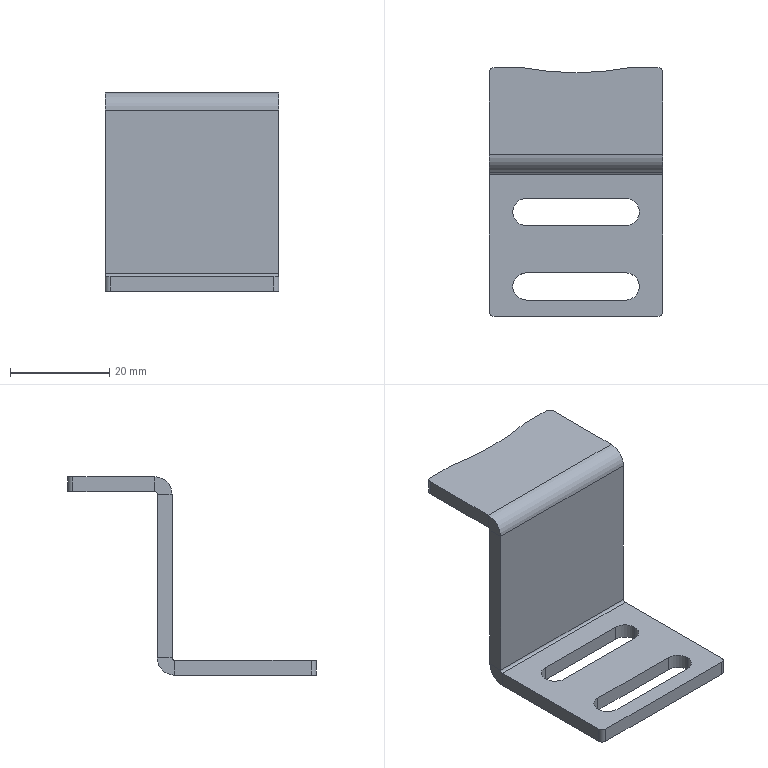Part | SolidWorks | features BaseBody 1 | 1 solid | 38 faces | box 35 x 50 x 40 mm | volume 8107 mm3 | plane 23 | cylinder 15 | commonest cylinder face diameters 5.5 x6 2 x4 1 x2 7 x2 112 x1
STEP:
#1=CARTESIAN_POINT('',(-10.536,34.,37.));
#2=VERTEX_POINT('',#1);
#3=CARTESIAN_POINT('',(10.536,34.,37.));
#4=VERTEX_POINT('',#3);
#5=CARTESIAN_POINT('',(0.,89.,37.));
#6=DIRECTION('',(0.,0.,1.));
#7=DIRECTION('',(-1.,0.,0.));
#8=AXIS2_PLACEMENT_3D('',#5,#6,#7);
#9=CIRCLE('',#8,56.);
#10=EDGE_CURVE('',#2,#4,#9,.T.);
#11=ORIENTED_EDGE('',*,*,#10,.T.);
#12=CARTESIAN_POINT('',(10.536,34.,34.));
#13=VERTEX_POINT('',#12);
#14=CARTESIAN_POINT('',(10.536,34.,37.));
#15=DIRECTION('',(0.,0.,-1.));
#16=VECTOR('',#15,1000.);
#17=LINE('',#14,#16);
#18=EDGE_CURVE('',#4,#13,#17,.T.);
#19=ORIENTED_EDGE('',*,*,#18,.T.);
#20=CARTESIAN_POINT('',(-10.536,34.,34.));
#21=VERTEX_POINT('',#20);
#22=CARTESIAN_POINT('',(0.,89.,34.));
#23=DIRECTION('',(0.,0.,1.));
#24=DIRECTION('',(-1.,0.,0.));
#25=AXIS2_PLACEMENT_3D('',#22,#23,#24);
#26=CIRCLE('',#25,56.);
#27=EDGE_CURVE('',#21,#13,#26,.T.);
#28=ORIENTED_EDGE('',*,*,#27,.F.);
#29=CARTESIAN_POINT('',(-10.536,34.,37.));
#30=DIRECTION('',(0.,0.,-1.));
#31=VECTOR('',#30,1000.);
#32=LINE('',#29,#31);
#33=EDGE_CURVE('',#2,#21,#32,.T.);
#34=ORIENTED_EDGE('',*,*,#33,.F.);
#35=EDGE_LOOP('',(#11,#19,#28,#34));
#36=FACE_OUTER_BOUND('',#35,.T.);
#37=CARTESIAN_POINT('',(0.,89.,37.));
#38=DIRECTION('',(0.,0.,-1.));
#39=DIRECTION('',(-1.,0.,0.));
#40=AXIS2_PLACEMENT_3D('',#37,#38,#39);
#41=CYLINDRICAL_SURFACE('',#40,56.);
#42=ADVANCED_FACE('',(#36),#41,.F.);
#43=CARTESIAN_POINT('',(17.5,-15.,-3.));
#44=VERTEX_POINT('',#43);
#45=CARTESIAN_POINT('',(16.5,-16.,-3.));
#46=VERTEX_POINT('',#45);
#47=CARTESIAN_POINT('',(16.5,-15.,-3.));
#48=DIRECTION('',(0.,0.,-1.));
#49=DIRECTION('',(1.,0.,0.));
#50=AXIS2_PLACEMENT_3D('',#47,#48,#49);
#51=CIRCLE('',#50,1.);
#52=EDGE_CURVE('',#44,#46,#51,.T.);
#53=ORIENTED_EDGE('',*,*,#52,.F.);
#54=CARTESIAN_POINT('',(17.5,-15.,0.));
#55=VERTEX_POINT('',#54);
#56=CARTESIAN_POINT('',(17.5,-15.,-3.));
#57=DIRECTION('',(0.,0.,-1.));
#58=VECTOR('',#57,1000.);
#59=LINE('',#56,#58);
#60=EDGE_CURVE('',#55,#44,#59,.T.);
#61=ORIENTED_EDGE('',*,*,#60,.F.);
#62=CARTESIAN_POINT('',(16.5,-16.,0.));
#63=VERTEX_POINT('',#62);
#64=CARTESIAN_POINT('',(16.5,-15.,0.));
#65=DIRECTION('',(0.,0.,1.));
#66=DIRECTION('',(1.,0.,0.));
#67=AXIS2_PLACEMENT_3D('',#64,#65,#66);
#68=CIRCLE('',#67,1.);
#69=EDGE_CURVE('',#63,#55,#68,.T.);
#70=ORIENTED_EDGE('',*,*,#69,.F.);
#71=CARTESIAN_POINT('',(16.5,-16.,-3.));
#72=DIRECTION('',(0.,0.,1.));
#73=VECTOR('',#72,1000.);
#74=LINE('',#71,#73);
#75=EDGE_CURVE('',#46,#63,#74,.T.);
#76=ORIENTED_EDGE('',*,*,#75,.F.);
#77=EDGE_LOOP('',(#53,#61,#70,#76));
#78=FACE_OUTER_BOUND('',#77,.T.);
#79=CARTESIAN_POINT('',(16.5,-15.,-3.));
#80=DIRECTION('',(0.,0.,1.));
#81=DIRECTION('',(1.,0.,0.));
#82=AXIS2_PLACEMENT_3D('',#79,#80,#81);
#83=CYLINDRICAL_SURFACE('',#82,1.);
#84=ADVANCED_FACE('',(#78),#83,.T.);
#85=CARTESIAN_POINT('',(-16.5,-16.,-3.));
#86=VERTEX_POINT('',#85);
#87=CARTESIAN_POINT('',(-17.5,-15.,-3.));
#88=VERTEX_POINT('',#87);
#89=CARTESIAN_POINT('',(-16.5,-15.,-3.));
#90=DIRECTION('',(0.,0.,-1.));
#91=DIRECTION('',(1.,0.,0.));
#92=AXIS2_PLACEMENT_3D('',#89,#90,#91);
#93=CIRCLE('',#92,1.);
#94=EDGE_CURVE('',#86,#88,#93,.T.);
#95=ORIENTED_EDGE('',*,*,#94,.F.);
#96=CARTESIAN_POINT('',(-16.5,-16.,0.));
#97=VERTEX_POINT('',#96);
#98=CARTESIAN_POINT('',(-16.5,-16.,-3.));
#99=DIRECTION('',(0.,0.,-1.));
#100=VECTOR('',#99,1000.);
#101=LINE('',#98,#100);
#102=EDGE_CURVE('',#97,#86,#101,.T.);
#103=ORIENTED_EDGE('',*,*,#102,.F.);
#104=CARTESIAN_POINT('',(-17.5,-15.,0.));
#105=VERTEX_POINT('',#104);
#106=CARTESIAN_POINT('',(-16.5,-15.,0.));
#107=DIRECTION('',(0.,0.,1.));
#108=DIRECTION('',(1.,0.,0.));
#109=AXIS2_PLACEMENT_3D('',#106,#107,#108);
#110=CIRCLE('',#109,1.);
#111=EDGE_CURVE('',#105,#97,#110,.T.);
#112=ORIENTED_EDGE('',*,*,#111,.F.);
#113=CARTESIAN_POINT('',(-17.5,-15.,-3.));
#114=DIRECTION('',(0.,0.,1.));
#115=VECTOR('',#114,1000.);
#116=LINE('',#113,#115);
#117=EDGE_CURVE('',#88,#105,#116,.T.);
#118=ORIENTED_EDGE('',*,*,#117,.F.);
#119=EDGE_LOOP('',(#95,#103,#112,#118));
#120=FACE_OUTER_BOUND('',#119,.T.);
#121=CARTESIAN_POINT('',(-16.5,-15.,-3.));
#122=DIRECTION('',(0.,0.,1.));
#123=DIRECTION('',(1.,0.,0.));
#124=AXIS2_PLACEMENT_3D('',#121,#122,#123);
#125=CYLINDRICAL_SURFACE('',#124,1.);
#126=ADVANCED_FACE('',(#120),#125,.T.);
#127=CARTESIAN_POINT('',(-16.5,34.,37.));
#128=VERTEX_POINT('',#127);
#129=CARTESIAN_POINT('',(-17.5,33.,37.));
#130=VERTEX_POINT('',#129);
#131=CARTESIAN_POINT('',(-16.5,33.,37.));
#132=DIRECTION('',(0.,0.,1.));
#133=DIRECTION('',(-1.,0.,0.));
#134=AXIS2_PLACEMENT_3D('',#131,#132,#133);
#135=CIRCLE('',#134,1.);
#136=EDGE_CURVE('',#128,#130,#135,.T.);
#137=ORIENTED_EDGE('',*,*,#136,.F.);
#138=CARTESIAN_POINT('',(-16.5,34.,34.));
#139=VERTEX_POINT('',#138);
#140=CARTESIAN_POINT('',(-16.5,34.,37.));
#141=DIRECTION('',(0.,0.,1.));
#142=VECTOR('',#141,1000.);
#143=LINE('',#140,#142);
#144=EDGE_CURVE('',#139,#128,#143,.T.);
#145=ORIENTED_EDGE('',*,*,#144,.F.);
#146=CARTESIAN_POINT('',(-17.5,33.,34.));
#147=VERTEX_POINT('',#146);
#148=CARTESIAN_POINT('',(-16.5,33.,34.));
#149=DIRECTION('',(0.,0.,-1.));
#150=DIRECTION('',(-1.,0.,0.));
#151=AXIS2_PLACEMENT_3D('',#148,#149,#150);
#152=CIRCLE('',#151,1.);
#153=EDGE_CURVE('',#147,#139,#152,.T.);
#154=ORIENTED_EDGE('',*,*,#153,.F.);
#155=CARTESIAN_POINT('',(-17.5,33.,37.));
#156=DIRECTION('',(0.,0.,-1.));
#157=VECTOR('',#156,1000.);
#158=LINE('',#155,#157);
#159=EDGE_CURVE('',#130,#147,#158,.T.);
#160=ORIENTED_EDGE('',*,*,#159,.F.);
#161=EDGE_LOOP('',(#137,#145,#154,#160));
#162=FACE_OUTER_BOUND('',#161,.T.);
#163=CARTESIAN_POINT('',(-16.5,33.,37.));
#164=DIRECTION('',(0.,0.,-1.));
#165=DIRECTION('',(-1.,0.,0.));
#166=AXIS2_PLACEMENT_3D('',#163,#164,#165);
#167=CYLINDRICAL_SURFACE('',#166,1.);
#168=ADVANCED_FACE('',(#162),#167,.T.);
#169=CARTESIAN_POINT('',(17.5,33.,37.));
#170=VERTEX_POINT('',#169);
#171=CARTESIAN_POINT('',(16.5,34.,37.));
#172=VERTEX_POINT('',#171);
#173=CARTESIAN_POINT('',(16.5,33.,37.));
#174=DIRECTION('',(0.,0.,1.));
#175=DIRECTION('',(-1.,0.,0.));
#176=AXIS2_PLACEMENT_3D('',#173,#174,#175);
#177=CIRCLE('',#176,1.);
#178=EDGE_CURVE('',#170,#172,#177,.T.);
#179=ORIENTED_EDGE('',*,*,#178,.F.);
#180=CARTESIAN_POINT('',(17.5,33.,34.));
#181=VERTEX_POINT('',#180);
#182=CARTESIAN_POINT('',(17.5,33.,37.));
#183=DIRECTION('',(0.,0.,1.));
#184=VECTOR('',#183,1000.);
#185=LINE('',#182,#184);
#186=EDGE_CURVE('',#181,#170,#185,.T.);
#187=ORIENTED_EDGE('',*,*,#186,.F.);
#188=CARTESIAN_POINT('',(16.5,34.,34.));
#189=VERTEX_POINT('',#188);
#190=CARTESIAN_POINT('',(16.5,33.,34.));
#191=DIRECTION('',(0.,0.,-1.));
#192=DIRECTION('',(-1.,0.,0.));
#193=AXIS2_PLACEMENT_3D('',#190,#191,#192);
#194=CIRCLE('',#193,1.);
#195=EDGE_CURVE('',#189,#181,#194,.T.);
#196=ORIENTED_EDGE('',*,*,#195,.F.);
#197=CARTESIAN_POINT('',(16.5,34.,37.));
#198=DIRECTION('',(0.,0.,-1.));
#199=VECTOR('',#198,1000.);
#200=LINE('',#197,#199);
#201=EDGE_CURVE('',#172,#189,#200,.T.);
#202=ORIENTED_EDGE('',*,*,#201,.F.);
#203=EDGE_LOOP('',(#179,#187,#196,#202));
#204=FACE_OUTER_BOUND('',#203,.T.);
#205=CARTESIAN_POINT('',(16.5,33.,37.));
#206=DIRECTION('',(0.,0.,-1.));
#207=DIRECTION('',(-1.,0.,0.));
#208=AXIS2_PLACEMENT_3D('',#205,#206,#207);
#209=CYLINDRICAL_SURFACE('',#208,1.);
#210=ADVANCED_FACE('',(#204),#209,.T.);
#211=CARTESIAN_POINT('',(-10.,-7.25,-3.));
#212=VERTEX_POINT('',#211);
#213=CARTESIAN_POINT('',(10.,-7.25,-3.));
#214=VERTEX_POINT('',#213);
#215=CARTESIAN_POINT('',(10.,-7.25,-3.));
#216=DIRECTION('',(1.,0.,0.));
#217=VECTOR('',#216,1000.);
#218=LINE('',#215,#217);
#219=EDGE_CURVE('',#212,#214,#218,.T.);
#220=ORIENTED_EDGE('',*,*,#219,.T.);
#221=CARTESIAN_POINT('',(10.,-7.25,0.));
#222=VERTEX_POINT('',#221);
#223=CARTESIAN_POINT('',(10.,-7.25,-3.001));
#224=DIRECTION('',(0.,0.,1.));
#225=VECTOR('',#224,1000.);
#226=LINE('',#223,#225);
#227=EDGE_CURVE('',#214,#222,#226,.T.);
#228=ORIENTED_EDGE('',*,*,#227,.T.);
#229=CARTESIAN_POINT('',(-10.,-7.25,0.));
#230=VERTEX_POINT('',#229);
#231=CARTESIAN_POINT('',(10.,-7.25,0.));
#232=DIRECTION('',(-1.,0.,0.));
#233=VECTOR('',#232,1000.);
#234=LINE('',#231,#233);
#235=EDGE_CURVE('',#222,#230,#234,.T.);
#236=ORIENTED_EDGE('',*,*,#235,.T.);
#237=CARTESIAN_POINT('',(-10.,-7.25,-3.001));
#238=DIRECTION('',(0.,0.,1.));
#239=VECTOR('',#238,1000.);
#240=LINE('',#237,#239);
#241=EDGE_CURVE('',#212,#230,#240,.T.);
#242=ORIENTED_EDGE('',*,*,#241,.F.);
#243=EDGE_LOOP('',(#220,#228,#236,#242));
#244=FACE_OUTER_BOUND('',#243,.T.);
#245=CARTESIAN_POINT('',(10.,-7.25,-3.001));
#246=DIRECTION('',(0.,1.,0.));
#247=DIRECTION('',(1.,0.,0.));
#248=AXIS2_PLACEMENT_3D('',#245,#246,#247);
#249=PLANE('',#248);
#250=ADVANCED_FACE('',(#244),#249,.F.);
#251=CARTESIAN_POINT('',(-10.,-12.75,-3.));
#252=VERTEX_POINT('',#251);
#253=CARTESIAN_POINT('',(-10.,-10.,-3.));
#254=DIRECTION('',(0.,0.,-1.));
#255=DIRECTION('',(1.,0.,0.));
#256=AXIS2_PLACEMENT_3D('',#253,#254,#255);
#257=CIRCLE('',#256,2.75);
#258=EDGE_CURVE('',#252,#212,#257,.T.);
#259=ORIENTED_EDGE('',*,*,#258,.T.);
#260=ORIENTED_EDGE('',*,*,#241,.T.);
#261=CARTESIAN_POINT('',(-10.,-12.75,0.));
#262=VERTEX_POINT('',#261);
#263=CARTESIAN_POINT('',(-10.,-10.,0.));
#264=DIRECTION('',(0.,0.,1.));
#265=DIRECTION('',(1.,0.,0.));
#266=AXIS2_PLACEMENT_3D('',#263,#264,#265);
#267=CIRCLE('',#266,2.75);
#268=EDGE_CURVE('',#230,#262,#267,.T.);
#269=ORIENTED_EDGE('',*,*,#268,.T.);
#270=CARTESIAN_POINT('',(-10.,-12.75,-3.001));
#271=DIRECTION('',(0.,0.,1.));
#272=VECTOR('',#271,1000.);
#273=LINE('',#270,#272);
#274=EDGE_CURVE('',#252,#262,#273,.T.);
#275=ORIENTED_EDGE('',*,*,#274,.F.);
#276=EDGE_LOOP('',(#259,#260,#269,#275));
#277=FACE_OUTER_BOUND('',#276,.T.);
#278=CARTESIAN_POINT('',(-10.,-10.,-3.001));
#279=DIRECTION('',(0.,0.,1.));
#280=DIRECTION('',(1.,0.,0.));
#281=AXIS2_PLACEMENT_3D('',#278,#279,#280);
#282=CYLINDRICAL_SURFACE('',#281,2.75);
#283=ADVANCED_FACE('',(#277),#282,.F.);
#284=CARTESIAN_POINT('',(10.,-12.75,-3.));
#285=VERTEX_POINT('',#284);
#286=CARTESIAN_POINT('',(10.,-12.75,-3.));
#287=DIRECTION('',(-1.,0.,0.));
#288=VECTOR('',#287,1000.);
#289=LINE('',#286,#288);
#290=EDGE_CURVE('',#285,#252,#289,.T.);
#291=ORIENTED_EDGE('',*,*,#290,.T.);
#292=ORIENTED_EDGE('',*,*,#274,.T.);
#293=CARTESIAN_POINT('',(10.,-12.75,0.));
#294=VERTEX_POINT('',#293);
#295=CARTESIAN_POINT('',(10.,-12.75,0.));
#296=DIRECTION('',(1.,0.,0.));
#297=VECTOR('',#296,1000.);
#298=LINE('',#295,#297);
#299=EDGE_CURVE('',#262,#294,#298,.T.);
#300=ORIENTED_EDGE('',*,*,#299,.T.);
#301=CARTESIAN_POINT('',(10.,-12.75,-3.001));
#302=DIRECTION('',(0.,0.,1.));
#303=VECTOR('',#302,1000.);
#304=LINE('',#301,#303);
#305=EDGE_CURVE('',#285,#294,#304,.T.);
#306=ORIENTED_EDGE('',*,*,#305,.F.);
#307=EDGE_LOOP('',(#291,#292,#300,#306));
#308=FACE_OUTER_BOUND('',#307,.T.);
#309=CARTESIAN_POINT('',(10.,-12.75,-3.001));
#310=DIRECTION('',(0.,-1.,0.));
#311=DIRECTION('',(0.,0.,-1.));
#312=AXIS2_PLACEMENT_3D('',#309,#310,#311);
#313=PLANE('',#312);
#314=ADVANCED_FACE('',(#308),#313,.F.);
#315=CARTESIAN_POINT('',(12.75,-10.,-3.));
#316=VERTEX_POINT('',#315);
#317=CARTESIAN_POINT('',(12.75,-10.,0.));
#318=VERTEX_POINT('',#317);
#319=CARTESIAN_POINT('',(12.75,-10.,-3.001));
#320=DIRECTION('',(0.,0.,1.));
#321=VECTOR('',#320,1000.);
#322=LINE('',#319,#321);
#323=EDGE_CURVE('',#316,#318,#322,.T.);
#324=ORIENTED_EDGE('',*,*,#323,.F.);
#325=CARTESIAN_POINT('',(10.,-10.,-3.));
#326=DIRECTION('',(0.,0.,-1.));
#327=DIRECTION('',(1.,0.,0.));
#328=AXIS2_PLACEMENT_3D('',#325,#326,#327);
#329=CIRCLE('',#328,2.75);
#330=EDGE_CURVE('',#316,#285,#329,.T.);
#331=ORIENTED_EDGE('',*,*,#330,.T.);
#332=ORIENTED_EDGE('',*,*,#305,.T.);
#333=CARTESIAN_POINT('',(10.,-10.,0.));
#334=DIRECTION('',(0.,0.,1.));
#335=DIRECTION('',(1.,0.,0.));
#336=AXIS2_PLACEMENT_3D('',#333,#334,#335);
#337=CIRCLE('',#336,2.75);
#338=EDGE_CURVE('',#294,#318,#337,.T.);
#339=ORIENTED_EDGE('',*,*,#338,.T.);
#340=EDGE_LOOP('',(#324,#331,#332,#339));
#341=FACE_OUTER_BOUND('',#340,.T.);
#342=CARTESIAN_POINT('',(10.,-10.,-3.001));
#343=DIRECTION('',(0.,0.,1.));
#344=DIRECTION('',(1.,0.,0.));
#345=AXIS2_PLACEMENT_3D('',#342,#343,#344);
#346=CYLINDRICAL_SURFACE('',#345,2.75);
#347=ADVANCED_FACE('',(#341),#346,.F.);
#348=CARTESIAN_POINT('',(-10.,7.75,-3.));
#349=VERTEX_POINT('',#348);
#350=CARTESIAN_POINT('',(10.,7.75,-3.));
#351=VERTEX_POINT('',#350);
#352=CARTESIAN_POINT('',(10.,7.75,-3.));
#353=DIRECTION('',(1.,0.,0.));
#354=VECTOR('',#353,1000.);
#355=LINE('',#352,#354);
#356=EDGE_CURVE('',#349,#351,#355,.T.);
#357=ORIENTED_EDGE('',*,*,#356,.T.);
#358=CARTESIAN_POINT('',(10.,7.75,0.));
#359=VERTEX_POINT('',#358);
#360=CARTESIAN_POINT('',(10.,7.75,-3.001));
#361=DIRECTION('',(0.,0.,1.));
#362=VECTOR('',#361,1000.);
#363=LINE('',#360,#362);
#364=EDGE_CURVE('',#351,#359,#363,.T.);
#365=ORIENTED_EDGE('',*,*,#364,.T.);
#366=CARTESIAN_POINT('',(-10.,7.75,0.));
#367=VERTEX_POINT('',#366);
#368=CARTESIAN_POINT('',(10.,7.75,0.));
#369=DIRECTION('',(-1.,0.,0.));
#370=VECTOR('',#369,1000.);
#371=LINE('',#368,#370);
#372=EDGE_CURVE('',#359,#367,#371,.T.);
#373=ORIENTED_EDGE('',*,*,#372,.T.);
#374=CARTESIAN_POINT('',(-10.,7.75,-3.001));
#375=DIRECTION('',(0.,0.,1.));
#376=VECTOR('',#375,1000.);
#377=LINE('',#374,#376);
#378=EDGE_CURVE('',#349,#367,#377,.T.);
#379=ORIENTED_EDGE('',*,*,#378,.F.);
#380=EDGE_LOOP('',(#357,#365,#373,#379));
#381=FACE_OUTER_BOUND('',#380,.T.);
#382=CARTESIAN_POINT('',(10.,7.75,-3.001));
#383=DIRECTION('',(0.,1.,0.));
#384=DIRECTION('',(1.,0.,0.));
#385=AXIS2_PLACEMENT_3D('',#382,#383,#384);
#386=PLANE('',#385);
#387=ADVANCED_FACE('',(#381),#386,.F.);
#388=CARTESIAN_POINT('',(-10.,2.25,-3.));
#389=VERTEX_POINT('',#388);
#390=CARTESIAN_POINT('',(-10.,5.,-3.));
#391=DIRECTION('',(0.,0.,-1.));
#392=DIRECTION('',(1.,0.,0.));
#393=AXIS2_PLACEMENT_3D('',#390,#391,#392);
#394=CIRCLE('',#393,2.75);
#395=EDGE_CURVE('',#389,#349,#394,.T.);
#396=ORIENTED_EDGE('',*,*,#395,.T.);
#397=ORIENTED_EDGE('',*,*,#378,.T.);
#398=CARTESIAN_POINT('',(-10.,2.25,0.));
#399=VERTEX_POINT('',#398);
#400=CARTESIAN_POINT('',(-10.,5.,0.));
#401=DIRECTION('',(0.,0.,1.));
#402=DIRECTION('',(1.,0.,0.));
#403=AXIS2_PLACEMENT_3D('',#400,#401,#402);
#404=CIRCLE('',#403,2.75);
#405=EDGE_CURVE('',#367,#399,#404,.T.);
#406=ORIENTED_EDGE('',*,*,#405,.T.);
#407=CARTESIAN_POINT('',(-10.,2.25,-3.001));
#408=DIRECTION('',(0.,0.,1.));
#409=VECTOR('',#408,1000.);
#410=LINE('',#407,#409);
#411=EDGE_CURVE('',#389,#399,#410,.T.);
#412=ORIENTED_EDGE('',*,*,#411,.F.);
#413=EDGE_LOOP('',(#396,#397,#406,#412));
#414=FACE_OUTER_BOUND('',#413,.T.);
#415=CARTESIAN_POINT('',(-10.,5.,-3.001));
#416=DIRECTION('',(0.,0.,1.));
#417=DIRECTION('',(1.,0.,0.));
#418=AXIS2_PLACEMENT_3D('',#415,#416,#417);
#419=CYLINDRICAL_SURFACE('',#418,2.75);
#420=ADVANCED_FACE('',(#414),#419,.F.);
#421=CARTESIAN_POINT('',(10.,2.25,-3.));
#422=VERTEX_POINT('',#421);
#423=CARTESIAN_POINT('',(10.,2.25,-3.));
#424=DIRECTION('',(-1.,0.,0.));
#425=VECTOR('',#424,1000.);
#426=LINE('',#423,#425);
#427=EDGE_CURVE('',#422,#389,#426,.T.);
#428=ORIENTED_EDGE('',*,*,#427,.T.);
#429=ORIENTED_EDGE('',*,*,#411,.T.);
#430=CARTESIAN_POINT('',(10.,2.25,0.));
#431=VERTEX_POINT('',#430);
#432=CARTESIAN_POINT('',(10.,2.25,0.));
#433=DIRECTION('',(1.,0.,0.));
#434=VECTOR('',#433,1000.);
#435=LINE('',#432,#434);
#436=EDGE_CURVE('',#399,#431,#435,.T.);
#437=ORIENTED_EDGE('',*,*,#436,.T.);
#438=CARTESIAN_POINT('',(10.,2.25,-3.001));
#439=DIRECTION('',(0.,0.,1.));
#440=VECTOR('',#439,1000.);
#441=LINE('',#438,#440);
#442=EDGE_CURVE('',#422,#431,#441,.T.);
#443=ORIENTED_EDGE('',*,*,#442,.F.);
#444=EDGE_LOOP('',(#428,#429,#437,#443));
#445=FACE_OUTER_BOUND('',#444,.T.);
#446=CARTESIAN_POINT('',(10.,2.25,-3.001));
#447=DIRECTION('',(0.,-1.,0.));
#448=DIRECTION('',(0.,0.,-1.));
#449=AXIS2_PLACEMENT_3D('',#446,#447,#448);
#450=PLANE('',#449);
#451=ADVANCED_FACE('',(#445),#450,.F.);
#452=CARTESIAN_POINT('',(12.75,5.,-3.));
#453=VERTEX_POINT('',#452);
#454=CARTESIAN_POINT('',(12.75,5.,0.));
#455=VERTEX_POINT('',#454);
#456=CARTESIAN_POINT('',(12.75,5.,-3.001));
#457=DIRECTION('',(0.,0.,1.));
#458=VECTOR('',#457,1000.);
#459=LINE('',#456,#458);
#460=EDGE_CURVE('',#453,#455,#459,.T.);
#461=ORIENTED_EDGE('',*,*,#460,.F.);
#462=CARTESIAN_POINT('',(10.,5.,-3.));
#463=DIRECTION('',(0.,0.,-1.));
#464=DIRECTION('',(1.,0.,0.));
#465=AXIS2_PLACEMENT_3D('',#462,#463,#464);
#466=CIRCLE('',#465,2.75);
#467=EDGE_CURVE('',#453,#422,#466,.T.);
#468=ORIENTED_EDGE('',*,*,#467,.T.);
#469=ORIENTED_EDGE('',*,*,#442,.T.);
#470=CARTESIAN_POINT('',(10.,5.,0.));
#471=DIRECTION('',(0.,0.,1.));
#472=DIRECTION('',(1.,0.,0.));
#473=AXIS2_PLACEMENT_3D('',#470,#471,#472);
#474=CIRCLE('',#473,2.75);
#475=EDGE_CURVE('',#431,#455,#474,.T.);
#476=ORIENTED_EDGE('',*,*,#475,.T.);
#477=EDGE_LOOP('',(#461,#468,#469,#476));
#478=FACE_OUTER_BOUND('',#477,.T.);
#479=CARTESIAN_POINT('',(10.,5.,-3.001));
#480=DIRECTION('',(0.,0.,1.));
#481=DIRECTION('',(1.,0.,0.));
#482=AXIS2_PLACEMENT_3D('',#479,#480,#481);
#483=CYLINDRICAL_SURFACE('',#482,2.75);
#484=ADVANCED_FACE('',(#478),#483,.F.);
#485=CARTESIAN_POINT('',(-17.5,34.,34.));
#486=DIRECTION('',(-1.,0.,0.));
#487=VECTOR('',#486,1000.);
#488=LINE('',#485,#487);
#489=EDGE_CURVE('',#21,#139,#488,.T.);
#490=ORIENTED_EDGE('',*,*,#489,.F.);
#491=ORIENTED_EDGE('',*,*,#27,.T.);
#492=CARTESIAN_POINT('',(-17.5,34.,34.));
#493=DIRECTION('',(-1.,0.,0.));
#494=VECTOR('',#493,1000.);
#495=LINE('',#492,#494);
#496=EDGE_CURVE('',#189,#13,#495,.T.);
#497=ORIENTED_EDGE('',*,*,#496,.F.);
#498=ORIENTED_EDGE('',*,*,#195,.T.);
#499=CARTESIAN_POINT('',(17.5,16.5,34.));
#500=VERTEX_POINT('',#499);
#501=CARTESIAN_POINT('',(17.5,34.,34.));
#502=DIRECTION('',(0.,1.,0.));
#503=VECTOR('',#502,1000.);
#504=LINE('',#501,#503);
#505=EDGE_CURVE('',#500,#181,#504,.T.);
#506=ORIENTED_EDGE('',*,*,#505,.F.);
#507=CARTESIAN_POINT('',(-17.5,16.5,34.));
#508=VERTEX_POINT('',#507);
#509=CARTESIAN_POINT('',(-17.5,16.5,34.));
#510=DIRECTION('',(1.,0.,0.));
#511=VECTOR('',#510,1000.);
#512=LINE('',#509,#511);
#513=EDGE_CURVE('',#508,#500,#512,.T.);
#514=ORIENTED_EDGE('',*,*,#513,.F.);
#515=CARTESIAN_POINT('',(-17.5,16.,34.));
#516=DIRECTION('',(0.,-1.,0.));
#517=VECTOR('',#516,1000.);
#518=LINE('',#515,#517);
#519=EDGE_CURVE('',#147,#508,#518,.T.);
#520=ORIENTED_EDGE('',*,*,#519,.F.);
#521=ORIENTED_EDGE('',*,*,#153,.T.);
#522=EDGE_LOOP('',(#490,#491,#497,#498,#506,#514,#520,#521));
#523=FACE_OUTER_BOUND('',#522,.T.);
#524=CARTESIAN_POINT('',(0.,0.,34.));
#525=DIRECTION('',(0.,0.,-1.));
#526=DIRECTION('',(0.,-1.,0.));
#527=AXIS2_PLACEMENT_3D('',#524,#525,#526);
#528=PLANE('',#527);
#529=ADVANCED_FACE('',(#523),#528,.T.);
#530=ORIENTED_EDGE('',*,*,#10,.F.);
#531=CARTESIAN_POINT('',(0.,34.,37.));
#532=DIRECTION('',(-1.,0.,0.));
#533=VECTOR('',#532,1000.);
#534=LINE('',#531,#533);
#535=EDGE_CURVE('',#2,#128,#534,.T.);
#536=ORIENTED_EDGE('',*,*,#535,.T.);
#537=ORIENTED_EDGE('',*,*,#136,.T.);
#538=CARTESIAN_POINT('',(-17.5,16.5,37.));
#539=VERTEX_POINT('',#538);
#540=CARTESIAN_POINT('',(-17.5,0.,37.));
#541=DIRECTION('',(0.,-1.,0.));
#542=VECTOR('',#541,1000.);
#543=LINE('',#540,#542);
#544=EDGE_CURVE('',#130,#539,#543,.T.);
#545=ORIENTED_EDGE('',*,*,#544,.T.);
#546=CARTESIAN_POINT('',(17.5,16.5,37.));
#547=VERTEX_POINT('',#546);
#548=CARTESIAN_POINT('',(-17.5,16.5,37.));
#549=DIRECTION('',(-1.,0.,0.));
#550=VECTOR('',#549,1000.);
#551=LINE('',#548,#550);
#552=EDGE_CURVE('',#547,#539,#551,.T.);
#553=ORIENTED_EDGE('',*,*,#552,.F.);
#554=CARTESIAN_POINT('',(17.5,0.,37.));
#555=DIRECTION('',(0.,1.,0.));
#556=VECTOR('',#555,1000.);
#557=LINE('',#554,#556);
#558=EDGE_CURVE('',#547,#170,#557,.T.);
#559=ORIENTED_EDGE('',*,*,#558,.T.);
#560=ORIENTED_EDGE('',*,*,#178,.T.);
#561=CARTESIAN_POINT('',(0.,34.,37.));
#562=DIRECTION('',(-1.,0.,0.));
#563=VECTOR('',#562,1000.);
#564=LINE('',#561,#563);
#565=EDGE_CURVE('',#172,#4,#564,.T.);
#566=ORIENTED_EDGE('',*,*,#565,.T.);
#567=EDGE_LOOP('',(#530,#536,#537,#545,#553,#559,#560,#566));
#568=FACE_OUTER_BOUND('',#567,.T.);
#569=CARTESIAN_POINT('',(0.,0.,37.));
#570=DIRECTION('',(0.,0.,-1.));
#571=DIRECTION('',(0.,-1.,0.));
#572=AXIS2_PLACEMENT_3D('',#569,#570,#571);
#573=PLANE('',#572);
#574=ADVANCED_FACE('',(#568),#573,.F.);
#575=ORIENTED_EDGE('',*,*,#505,.T.);
#576=ORIENTED_EDGE('',*,*,#186,.T.);
#577=ORIENTED_EDGE('',*,*,#558,.F.);
#578=CARTESIAN_POINT('',(17.5,16.5,34.));
#579=DIRECTION('',(0.,0.,1.));
#580=VECTOR('',#579,1000.);
#581=LINE('',#578,#580);
#582=EDGE_CURVE('',#500,#547,#581,.T.);
#583=ORIENTED_EDGE('',*,*,#582,.F.);
#584=EDGE_LOOP('',(#575,#576,#577,#583));
#585=FACE_OUTER_BOUND('',#584,.T.);
#586=CARTESIAN_POINT('',(17.5,34.,37.));
#587=DIRECTION('',(-1.,0.,0.));
#588=DIRECTION('',(0.,1.,0.));
#589=AXIS2_PLACEMENT_3D('',#586,#587,#588);
#590=PLANE('',#589);
#591=ADVANCED_FACE('',(#585),#590,.F.);
#592=ORIENTED_EDGE('',*,*,#544,.F.);
#593=ORIENTED_EDGE('',*,*,#159,.T.);
#594=ORIENTED_EDGE('',*,*,#519,.T.);
#595=CARTESIAN_POINT('',(-17.5,16.5,37.));
#596=DIRECTION('',(0.,0.,1.));
#597=VECTOR('',#596,1000.);
#598=LINE('',#595,#597);
#599=EDGE_CURVE('',#508,#539,#598,.T.);
#600=ORIENTED_EDGE('',*,*,#599,.T.);
#601=EDGE_LOOP('',(#592,#593,#594,#600));
#602=FACE_OUTER_BOUND('',#601,.T.);
#603=CARTESIAN_POINT('',(-17.5,16.,37.));
#604=DIRECTION('',(1.,0.,0.));
#605=DIRECTION('',(0.,1.,0.));
#606=AXIS2_PLACEMENT_3D('',#603,#604,#605);
#607=PLANE('',#606);
#608=ADVANCED_FACE('',(#602),#607,.F.);
#609=CARTESIAN_POINT('',(17.5,16.,33.5));
#610=VERTEX_POINT('',#609);
#611=CARTESIAN_POINT('',(-17.5,16.,33.5));
#612=VERTEX_POINT('',#611);
#613=CARTESIAN_POINT('',(17.5,16.,33.5));
#614=DIRECTION('',(-1.,0.,0.));
#615=VECTOR('',#614,1000.);
#616=LINE('',#613,#615);
#617=EDGE_CURVE('',#610,#612,#616,.T.);
#618=ORIENTED_EDGE('',*,*,#617,.T.);
#619=CARTESIAN_POINT('',(-17.5,16.5,33.5));
#620=DIRECTION('',(-1.,0.,0.));
#621=DIRECTION('',(0.,0.,-1.));
#622=AXIS2_PLACEMENT_3D('',#619,#620,#621);
#623=CIRCLE('',#622,0.5);
#624=EDGE_CURVE('',#612,#508,#623,.T.);
#625=ORIENTED_EDGE('',*,*,#624,.T.);
#626=ORIENTED_EDGE('',*,*,#513,.T.);
#627=CARTESIAN_POINT('',(17.5,16.5,33.5));
#628=DIRECTION('',(1.,0.,0.));
#629=DIRECTION('',(0.,0.,-1.));
#630=AXIS2_PLACEMENT_3D('',#627,#628,#629);
#631=CIRCLE('',#630,0.5);
#632=EDGE_CURVE('',#500,#610,#631,.T.);
#633=ORIENTED_EDGE('',*,*,#632,.T.);
#634=EDGE_LOOP('',(#618,#625,#626,#633));
#635=FACE_OUTER_BOUND('',#634,.T.);
#636=CARTESIAN_POINT('',(17.5,16.5,33.5));
#637=DIRECTION('',(1.,0.,0.));
#638=DIRECTION('',(0.,0.,1.));
#639=AXIS2_PLACEMENT_3D('',#636,#637,#638);
#640=CYLINDRICAL_SURFACE('',#639,0.5);
#641=ADVANCED_FACE('',(#635),#640,.F.);
#642=CARTESIAN_POINT('',(17.5,13.,33.5));
#643=VERTEX_POINT('',#642);
#644=CARTESIAN_POINT('',(-17.5,13.,33.5));
#645=VERTEX_POINT('',#644);
#646=CARTESIAN_POINT('',(17.5,13.,33.5));
#647=DIRECTION('',(-1.,0.,0.));
#648=VECTOR('',#647,1000.);
#649=LINE('',#646,#648);
#650=EDGE_CURVE('',#643,#645,#649,.T.);
#651=ORIENTED_EDGE('',*,*,#650,.F.);
#652=CARTESIAN_POINT('',(17.5,16.5,33.5));
#653=DIRECTION('',(1.,0.,0.));
#654=DIRECTION('',(0.,0.,-1.));
#655=AXIS2_PLACEMENT_3D('',#652,#653,#654);
#656=CIRCLE('',#655,3.5);
#657=EDGE_CURVE('',#547,#643,#656,.T.);
#658=ORIENTED_EDGE('',*,*,#657,.F.);
#659=ORIENTED_EDGE('',*,*,#552,.T.);
#660=CARTESIAN_POINT('',(-17.5,16.5,33.5));
#661=DIRECTION('',(-1.,0.,0.));
#662=DIRECTION('',(0.,0.,-1.));
#663=AXIS2_PLACEMENT_3D('',#660,#661,#662);
#664=CIRCLE('',#663,3.5);
#665=EDGE_CURVE('',#645,#539,#664,.T.);
#666=ORIENTED_EDGE('',*,*,#665,.F.);
#667=EDGE_LOOP('',(#651,#658,#659,#666));
#668=FACE_OUTER_BOUND('',#667,.T.);
#669=CARTESIAN_POINT('',(17.5,16.5,33.5));
#670=DIRECTION('',(1.,0.,0.));
#671=DIRECTION('',(0.,0.,1.));
#672=AXIS2_PLACEMENT_3D('',#669,#670,#671);
#673=CYLINDRICAL_SURFACE('',#672,3.5);
#674=ADVANCED_FACE('',(#668),#673,.T.);
#675=ORIENTED_EDGE('',*,*,#632,.F.);
#676=ORIENTED_EDGE('',*,*,#582,.T.);
#677=ORIENTED_EDGE('',*,*,#657,.T.);
#678=CARTESIAN_POINT('',(17.5,16.,33.5));
#679=DIRECTION('',(0.,-1.,0.));
#680=VECTOR('',#679,1000.);
#681=LINE('',#678,#680);
#682=EDGE_CURVE('',#610,#643,#681,.T.);
#683=ORIENTED_EDGE('',*,*,#682,.F.);
#684=EDGE_LOOP('',(#675,#676,#677,#683));
#685=FACE_OUTER_BOUND('',#684,.T.);
#686=CARTESIAN_POINT('',(17.5,16.5,33.5));
#687=DIRECTION('',(-1.,0.,0.));
#688=DIRECTION('',(0.,0.,1.));
#689=AXIS2_PLACEMENT_3D('',#686,#687,#688);
#690=PLANE('',#689);
#691=ADVANCED_FACE('',(#685),#690,.F.);
#692=ORIENTED_EDGE('',*,*,#599,.F.);
#693=ORIENTED_EDGE('',*,*,#624,.F.);
#694=CARTESIAN_POINT('',(-17.5,16.,33.5));
#695=DIRECTION('',(0.,-1.,0.));
#696=VECTOR('',#695,1000.);
#697=LINE('',#694,#696);
#698=EDGE_CURVE('',#612,#645,#697,.T.);
#699=ORIENTED_EDGE('',*,*,#698,.T.);
#700=ORIENTED_EDGE('',*,*,#665,.T.);
#701=EDGE_LOOP('',(#692,#693,#699,#700));
#702=FACE_OUTER_BOUND('',#701,.T.);
#703=CARTESIAN_POINT('',(-17.5,16.5,33.5));
#704=DIRECTION('',(-1.,0.,0.));
#705=DIRECTION('',(0.,0.,1.));
#706=AXIS2_PLACEMENT_3D('',#703,#704,#705);
#707=PLANE('',#706);
#708=ADVANCED_FACE('',(#702),#707,.T.);
#709=CARTESIAN_POINT('',(-17.5,12.5,0.));
#710=VERTEX_POINT('',#709);
#711=CARTESIAN_POINT('',(17.5,12.5,0.));
#712=VERTEX_POINT('',#711);
#713=CARTESIAN_POINT('',(-17.5,12.5,0.));
#714=DIRECTION('',(1.,0.,0.));
#715=VECTOR('',#714,1000.);
#716=LINE('',#713,#715);
#717=EDGE_CURVE('',#710,#712,#716,.T.);
#718=ORIENTED_EDGE('',*,*,#717,.T.);
#719=CARTESIAN_POINT('',(17.5,13.,0.5));
#720=VERTEX_POINT('',#719);
#721=CARTESIAN_POINT('',(17.5,12.5,0.5));
#722=DIRECTION('',(1.,0.,0.));
#723=DIRECTION('',(0.,0.,1.));
#724=AXIS2_PLACEMENT_3D('',#721,#722,#723);
#725=CIRCLE('',#724,0.5);
#726=EDGE_CURVE('',#712,#720,#725,.T.);
#727=ORIENTED_EDGE('',*,*,#726,.T.);
#728=CARTESIAN_POINT('',(-17.5,13.,0.5));
#729=VERTEX_POINT('',#728);
#730=CARTESIAN_POINT('',(17.5,13.,0.5));
#731=DIRECTION('',(-1.,0.,0.));
#732=VECTOR('',#731,1000.);
#733=LINE('',#730,#732);
#734=EDGE_CURVE('',#720,#729,#733,.T.);
#735=ORIENTED_EDGE('',*,*,#734,.T.);
#736=CARTESIAN_POINT('',(-17.5,12.5,0.5));
#737=DIRECTION('',(-1.,0.,0.));
#738=DIRECTION('',(0.,0.,1.));
#739=AXIS2_PLACEMENT_3D('',#736,#737,#738);
#740=CIRCLE('',#739,0.5);
#741=EDGE_CURVE('',#729,#710,#740,.T.);
#742=ORIENTED_EDGE('',*,*,#741,.T.);
#743=EDGE_LOOP('',(#718,#727,#735,#742));
#744=FACE_OUTER_BOUND('',#743,.T.);
#745=CARTESIAN_POINT('',(-17.5,12.5,0.5));
#746=DIRECTION('',(-1.,0.,0.));
#747=DIRECTION('',(0.,1.,0.));
#748=AXIS2_PLACEMENT_3D('',#745,#746,#747);
#749=CYLINDRICAL_SURFACE('',#748,0.5);
#750=ADVANCED_FACE('',(#744),#749,.F.);
#751=CARTESIAN_POINT('',(-17.5,12.5,-3.));
#752=VERTEX_POINT('',#751);
#753=CARTESIAN_POINT('',(17.5,12.5,-3.));
#754=VERTEX_POINT('',#753);
#755=CARTESIAN_POINT('',(-17.5,12.5,-3.));
#756=DIRECTION('',(1.,0.,0.));
#757=VECTOR('',#756,1000.);
#758=LINE('',#755,#757);
#759=EDGE_CURVE('',#752,#754,#758,.T.);
#760=ORIENTED_EDGE('',*,*,#759,.F.);
#761=CARTESIAN_POINT('',(-17.5,16.,0.5));
#762=VERTEX_POINT('',#761);
#763=CARTESIAN_POINT('',(-17.5,12.5,0.5));
#764=DIRECTION('',(-1.,0.,0.));
#765=DIRECTION('',(0.,0.,1.));
#766=AXIS2_PLACEMENT_3D('',#763,#764,#765);
#767=CIRCLE('',#766,3.5);
#768=EDGE_CURVE('',#762,#752,#767,.T.);
#769=ORIENTED_EDGE('',*,*,#768,.F.);
#770=CARTESIAN_POINT('',(17.5,16.,0.5));
#771=VERTEX_POINT('',#770);
#772=CARTESIAN_POINT('',(17.5,16.,0.5));
#773=DIRECTION('',(1.,0.,0.));
#774=VECTOR('',#773,1000.);
#775=LINE('',#772,#774);
#776=EDGE_CURVE('',#762,#771,#775,.T.);
#777=ORIENTED_EDGE('',*,*,#776,.T.);
#778=CARTESIAN_POINT('',(17.5,12.5,0.5));
#779=DIRECTION('',(1.,0.,0.));
#780=DIRECTION('',(0.,0.,1.));
#781=AXIS2_PLACEMENT_3D('',#778,#779,#780);
#782=CIRCLE('',#781,3.5);
#783=EDGE_CURVE('',#754,#771,#782,.T.);
#784=ORIENTED_EDGE('',*,*,#783,.F.);
#785=EDGE_LOOP('',(#760,#769,#777,#784));
#786=FACE_OUTER_BOUND('',#785,.T.);
#787=CARTESIAN_POINT('',(-17.5,12.5,0.5));
#788=DIRECTION('',(-1.,0.,0.));
#789=DIRECTION('',(0.,1.,0.));
#790=AXIS2_PLACEMENT_3D('',#787,#788,#789);
#791=CYLINDRICAL_SURFACE('',#790,3.5);
#792=ADVANCED_FACE('',(#786),#791,.T.);
#793=ORIENTED_EDGE('',*,*,#741,.F.);
#794=CARTESIAN_POINT('',(-17.5,13.,0.5));
#795=DIRECTION('',(0.,1.,0.));
#796=VECTOR('',#795,1000.);
#797=LINE('',#794,#796);
#798=EDGE_CURVE('',#729,#762,#797,.T.);
#799=ORIENTED_EDGE('',*,*,#798,.T.);
#800=ORIENTED_EDGE('',*,*,#768,.T.);
#801=CARTESIAN_POINT('',(-17.5,12.5,0.));
#802=DIRECTION('',(0.,0.,-1.));
#803=VECTOR('',#802,1000.);
#804=LINE('',#801,#803);
#805=EDGE_CURVE('',#710,#752,#804,.T.);
#806=ORIENTED_EDGE('',*,*,#805,.F.);
#807=EDGE_LOOP('',(#793,#799,#800,#806));
#808=FACE_OUTER_BOUND('',#807,.T.);
#809=CARTESIAN_POINT('',(-17.5,12.5,0.5));
#810=DIRECTION('',(1.,0.,0.));
#811=DIRECTION('',(0.,1.,0.));
#812=AXIS2_PLACEMENT_3D('',#809,#810,#811);
#813=PLANE('',#812);
#814=ADVANCED_FACE('',(#808),#813,.F.);
#815=CARTESIAN_POINT('',(17.5,16.,0.5));
#816=DIRECTION('',(0.,1.,0.));
#817=VECTOR('',#816,1000.);
#818=LINE('',#815,#817);
#819=EDGE_CURVE('',#720,#771,#818,.T.);
#820=ORIENTED_EDGE('',*,*,#819,.F.);
#821=ORIENTED_EDGE('',*,*,#726,.F.);
#822=CARTESIAN_POINT('',(17.5,12.5,0.));
#823=DIRECTION('',(0.,0.,-1.));
#824=VECTOR('',#823,1000.);
#825=LINE('',#822,#824);
#826=EDGE_CURVE('',#712,#754,#825,.T.);
#827=ORIENTED_EDGE('',*,*,#826,.T.);
#828=ORIENTED_EDGE('',*,*,#783,.T.);
#829=EDGE_LOOP('',(#820,#821,#827,#828));
#830=FACE_OUTER_BOUND('',#829,.T.);
#831=CARTESIAN_POINT('',(17.5,12.5,0.5));
#832=DIRECTION('',(1.,0.,0.));
#833=DIRECTION('',(0.,1.,0.));
#834=AXIS2_PLACEMENT_3D('',#831,#832,#833);
#835=PLANE('',#834);
#836=ADVANCED_FACE('',(#830),#835,.T.);
#837=CARTESIAN_POINT('',(17.5,-16.,0.));
#838=DIRECTION('',(1.,0.,0.));
#839=VECTOR('',#838,1000.);
#840=LINE('',#837,#839);
#841=EDGE_CURVE('',#97,#63,#840,.T.);
#842=ORIENTED_EDGE('',*,*,#841,.F.);
#843=ORIENTED_EDGE('',*,*,#102,.T.);
#844=CARTESIAN_POINT('',(17.5,-16.,-3.));
#845=DIRECTION('',(1.,0.,0.));
#846=VECTOR('',#845,1000.);
#847=LINE('',#844,#846);
#848=EDGE_CURVE('',#86,#46,#847,.T.);
#849=ORIENTED_EDGE('',*,*,#848,.T.);
#850=ORIENTED_EDGE('',*,*,#75,.T.);
#851=EDGE_LOOP('',(#842,#843,#849,#850));
#852=FACE_OUTER_BOUND('',#851,.T.);
#853=CARTESIAN_POINT('',(17.5,-16.,-3.));
#854=DIRECTION('',(0.,-1.,0.));
#855=DIRECTION('',(0.,0.,-1.));
#856=AXIS2_PLACEMENT_3D('',#853,#854,#855);
#857=PLANE('',#856);
#858=ADVANCED_FACE('',(#852),#857,.T.);
#859=CARTESIAN_POINT('',(17.5,-16.,0.));
#860=DIRECTION('',(0.,1.,0.));
#861=VECTOR('',#860,1000.);
#862=LINE('',#859,#861);
#863=EDGE_CURVE('',#55,#712,#862,.T.);
#864=ORIENTED_EDGE('',*,*,#863,.F.);
#865=ORIENTED_EDGE('',*,*,#60,.T.);
#866=CARTESIAN_POINT('',(17.5,-16.,-3.));
#867=DIRECTION('',(0.,1.,0.));
#868=VECTOR('',#867,1000.);
#869=LINE('',#866,#868);
#870=EDGE_CURVE('',#44,#754,#869,.T.);
#871=ORIENTED_EDGE('',*,*,#870,.T.);
#872=ORIENTED_EDGE('',*,*,#826,.F.);
#873=EDGE_LOOP('',(#864,#865,#871,#872));
#874=FACE_OUTER_BOUND('',#873,.T.);
#875=CARTESIAN_POINT('',(17.5,-16.,-3.));
#876=DIRECTION('',(1.,0.,0.));
#877=DIRECTION('',(0.,1.,0.));
#878=AXIS2_PLACEMENT_3D('',#875,#876,#877);
#879=PLANE('',#878);
#880=ADVANCED_FACE('',(#874),#879,.T.);
#881=ORIENTED_EDGE('',*,*,#475,.F.);
#882=ORIENTED_EDGE('',*,*,#436,.F.);
#883=ORIENTED_EDGE('',*,*,#405,.F.);
#884=ORIENTED_EDGE('',*,*,#372,.F.);
#885=CARTESIAN_POINT('',(10.,5.,0.));
#886=DIRECTION('',(0.,0.,1.));
#887=DIRECTION('',(1.,0.,0.));
#888=AXIS2_PLACEMENT_3D('',#885,#886,#887);
#889=CIRCLE('',#888,2.75);
#890=EDGE_CURVE('',#455,#359,#889,.T.);
#891=ORIENTED_EDGE('',*,*,#890,.F.);
#892=EDGE_LOOP('',(#881,#882,#883,#884,#891));
#893=FACE_BOUND('',#892,.T.);
#894=ORIENTED_EDGE('',*,*,#338,.F.);
#895=ORIENTED_EDGE('',*,*,#299,.F.);
#896=ORIENTED_EDGE('',*,*,#268,.F.);
#897=ORIENTED_EDGE('',*,*,#235,.F.);
#898=CARTESIAN_POINT('',(10.,-10.,0.));
#899=DIRECTION('',(0.,0.,1.));
#900=DIRECTION('',(1.,0.,0.));
#901=AXIS2_PLACEMENT_3D('',#898,#899,#900);
#902=CIRCLE('',#901,2.75);
#903=EDGE_CURVE('',#318,#222,#902,.T.);
#904=ORIENTED_EDGE('',*,*,#903,.F.);
#905=EDGE_LOOP('',(#894,#895,#896,#897,#904));
#906=FACE_BOUND('',#905,.T.);
#907=CARTESIAN_POINT('',(-17.5,-16.,0.));
#908=DIRECTION('',(0.,-1.,0.));
#909=VECTOR('',#908,1000.);
#910=LINE('',#907,#909);
#911=EDGE_CURVE('',#710,#105,#910,.T.);
#912=ORIENTED_EDGE('',*,*,#911,.T.);
#913=ORIENTED_EDGE('',*,*,#111,.T.);
#914=ORIENTED_EDGE('',*,*,#841,.T.);
#915=ORIENTED_EDGE('',*,*,#69,.T.);
#916=ORIENTED_EDGE('',*,*,#863,.T.);
#917=ORIENTED_EDGE('',*,*,#717,.F.);
#918=EDGE_LOOP('',(#912,#913,#914,#915,#916,#917));
#919=FACE_OUTER_BOUND('',#918,.T.);
#920=CARTESIAN_POINT('',(0.,0.,0.));
#921=DIRECTION('',(0.,0.,1.));
#922=DIRECTION('',(1.,0.,0.));
#923=AXIS2_PLACEMENT_3D('',#920,#921,#922);
#924=PLANE('',#923);
#925=ADVANCED_FACE('',(#893,#906,#919),#924,.T.);
#926=ORIENTED_EDGE('',*,*,#427,.F.);
#927=ORIENTED_EDGE('',*,*,#467,.F.);
#928=CARTESIAN_POINT('',(10.,5.,-3.));
#929=DIRECTION('',(0.,0.,-1.));
#930=DIRECTION('',(1.,0.,0.));
#931=AXIS2_PLACEMENT_3D('',#928,#929,#930);
#932=CIRCLE('',#931,2.75);
#933=EDGE_CURVE('',#351,#453,#932,.T.);
#934=ORIENTED_EDGE('',*,*,#933,.F.);
#935=ORIENTED_EDGE('',*,*,#356,.F.);
#936=ORIENTED_EDGE('',*,*,#395,.F.);
#937=EDGE_LOOP('',(#926,#927,#934,#935,#936));
#938=FACE_BOUND('',#937,.T.);
#939=ORIENTED_EDGE('',*,*,#290,.F.);
#940=ORIENTED_EDGE('',*,*,#330,.F.);
#941=CARTESIAN_POINT('',(10.,-10.,-3.));
#942=DIRECTION('',(0.,0.,-1.));
#943=DIRECTION('',(1.,0.,0.));
#944=AXIS2_PLACEMENT_3D('',#941,#942,#943);
#945=CIRCLE('',#944,2.75);
#946=EDGE_CURVE('',#214,#316,#945,.T.);
#947=ORIENTED_EDGE('',*,*,#946,.F.);
#948=ORIENTED_EDGE('',*,*,#219,.F.);
#949=ORIENTED_EDGE('',*,*,#258,.F.);
#950=EDGE_LOOP('',(#939,#940,#947,#948,#949));
#951=FACE_BOUND('',#950,.T.);
#952=ORIENTED_EDGE('',*,*,#848,.F.);
#953=ORIENTED_EDGE('',*,*,#94,.T.);
#954=CARTESIAN_POINT('',(-17.5,-16.,-3.));
#955=DIRECTION('',(0.,-1.,0.));
#956=VECTOR('',#955,1000.);
#957=LINE('',#954,#956);
#958=EDGE_CURVE('',#752,#88,#957,.T.);
#959=ORIENTED_EDGE('',*,*,#958,.F.);
#960=ORIENTED_EDGE('',*,*,#759,.T.);
#961=ORIENTED_EDGE('',*,*,#870,.F.);
#962=ORIENTED_EDGE('',*,*,#52,.T.);
#963=EDGE_LOOP('',(#952,#953,#959,#960,#961,#962));
#964=FACE_OUTER_BOUND('',#963,.T.);
#965=CARTESIAN_POINT('',(0.,0.,-3.));
#966=DIRECTION('',(0.,0.,1.));
#967=DIRECTION('',(1.,0.,0.));
#968=AXIS2_PLACEMENT_3D('',#965,#966,#967);
#969=PLANE('',#968);
#970=ADVANCED_FACE('',(#938,#951,#964),#969,.F.);
#971=ORIENTED_EDGE('',*,*,#958,.T.);
#972=ORIENTED_EDGE('',*,*,#117,.T.);
#973=ORIENTED_EDGE('',*,*,#911,.F.);
#974=ORIENTED_EDGE('',*,*,#805,.T.);
#975=EDGE_LOOP('',(#971,#972,#973,#974));
#976=FACE_OUTER_BOUND('',#975,.T.);
#977=CARTESIAN_POINT('',(-17.5,-16.,-3.));
#978=DIRECTION('',(-1.,0.,0.));
#979=DIRECTION('',(0.,0.,1.));
#980=AXIS2_PLACEMENT_3D('',#977,#978,#979);
#981=PLANE('',#980);
#982=ADVANCED_FACE('',(#976),#981,.T.);
#983=CARTESIAN_POINT('',(17.5,13.,0.));
#984=DIRECTION('',(0.,0.,-1.));
#985=VECTOR('',#984,1000.);
#986=LINE('',#983,#985);
#987=EDGE_CURVE('',#643,#720,#986,.T.);
#988=ORIENTED_EDGE('',*,*,#987,.F.);
#989=ORIENTED_EDGE('',*,*,#650,.T.);
#990=CARTESIAN_POINT('',(-17.5,13.,37.));
#991=DIRECTION('',(0.,0.,1.));
#992=VECTOR('',#991,1000.);
#993=LINE('',#990,#992);
#994=EDGE_CURVE('',#729,#645,#993,.T.);
#995=ORIENTED_EDGE('',*,*,#994,.F.);
#996=ORIENTED_EDGE('',*,*,#734,.F.);
#997=EDGE_LOOP('',(#988,#989,#995,#996));
#998=FACE_OUTER_BOUND('',#997,.T.);
#999=CARTESIAN_POINT('',(0.,13.,0.));
#1000=DIRECTION('',(0.,-1.,0.));
#1001=DIRECTION('',(-1.,0.,0.));
#1002=AXIS2_PLACEMENT_3D('',#999,#1000,#1001);
#1003=PLANE('',#1002);
#1004=ADVANCED_FACE('',(#998),#1003,.T.);
#1005=ORIENTED_EDGE('',*,*,#617,.F.);
#1006=CARTESIAN_POINT('',(17.5,16.,0.));
#1007=DIRECTION('',(0.,0.,-1.));
#1008=VECTOR('',#1007,1000.);
#1009=LINE('',#1006,#1008);
#1010=EDGE_CURVE('',#610,#771,#1009,.T.);
#1011=ORIENTED_EDGE('',*,*,#1010,.T.);
#1012=ORIENTED_EDGE('',*,*,#776,.F.);
#1013=CARTESIAN_POINT('',(-17.5,16.,0.));
#1014=DIRECTION('',(0.,0.,1.));
#1015=VECTOR('',#1014,1000.);
#1016=LINE('',#1013,#1015);
#1017=EDGE_CURVE('',#762,#612,#1016,.T.);
#1018=ORIENTED_EDGE('',*,*,#1017,.T.);
#1019=EDGE_LOOP('',(#1005,#1011,#1012,#1018));
#1020=FACE_OUTER_BOUND('',#1019,.T.);
#1021=CARTESIAN_POINT('',(0.,16.,0.));
#1022=DIRECTION('',(0.,-1.,0.));
#1023=DIRECTION('',(-1.,0.,0.));
#1024=AXIS2_PLACEMENT_3D('',#1021,#1022,#1023);
#1025=PLANE('',#1024);
#1026=ADVANCED_FACE('',(#1020),#1025,.F.);
#1027=ORIENTED_EDGE('',*,*,#698,.F.);
#1028=ORIENTED_EDGE('',*,*,#1017,.F.);
#1029=ORIENTED_EDGE('',*,*,#798,.F.);
#1030=ORIENTED_EDGE('',*,*,#994,.T.);
#1031=EDGE_LOOP('',(#1027,#1028,#1029,#1030));
#1032=FACE_OUTER_BOUND('',#1031,.T.);
#1033=CARTESIAN_POINT('',(-17.5,16.,37.));
#1034=DIRECTION('',(1.,0.,0.));
#1035=DIRECTION('',(0.,1.,0.));
#1036=AXIS2_PLACEMENT_3D('',#1033,#1034,#1035);
#1037=PLANE('',#1036);
#1038=ADVANCED_FACE('',(#1032),#1037,.F.);
#1039=ORIENTED_EDGE('',*,*,#682,.T.);
#1040=ORIENTED_EDGE('',*,*,#987,.T.);
#1041=ORIENTED_EDGE('',*,*,#819,.T.);
#1042=ORIENTED_EDGE('',*,*,#1010,.F.);
#1043=EDGE_LOOP('',(#1039,#1040,#1041,#1042));
#1044=FACE_OUTER_BOUND('',#1043,.T.);
#1045=CARTESIAN_POINT('',(17.5,16.,0.));
#1046=DIRECTION('',(-1.,0.,0.));
#1047=DIRECTION('',(0.,1.,0.));
#1048=AXIS2_PLACEMENT_3D('',#1045,#1046,#1047);
#1049=PLANE('',#1048);
#1050=ADVANCED_FACE('',(#1044),#1049,.F.);
#1051=ORIENTED_EDGE('',*,*,#18,.F.);
#1052=ORIENTED_EDGE('',*,*,#565,.F.);
#1053=ORIENTED_EDGE('',*,*,#201,.T.);
#1054=ORIENTED_EDGE('',*,*,#496,.T.);
#1055=EDGE_LOOP('',(#1051,#1052,#1053,#1054));
#1056=FACE_OUTER_BOUND('',#1055,.T.);
#1057=CARTESIAN_POINT('',(-17.5,34.,37.));
#1058=DIRECTION('',(0.,-1.,0.));
#1059=DIRECTION('',(0.,0.,-1.));
#1060=AXIS2_PLACEMENT_3D('',#1057,#1058,#1059);
#1061=PLANE('',#1060);
#1062=ADVANCED_FACE('',(#1056),#1061,.F.);
#1063=ORIENTED_EDGE('',*,*,#33,.T.);
#1064=ORIENTED_EDGE('',*,*,#489,.T.);
#1065=ORIENTED_EDGE('',*,*,#144,.T.);
#1066=ORIENTED_EDGE('',*,*,#535,.F.);
#1067=EDGE_LOOP('',(#1063,#1064,#1065,#1066));
#1068=FACE_OUTER_BOUND('',#1067,.T.);
#1069=CARTESIAN_POINT('',(-17.5,34.,37.));
#1070=DIRECTION('',(0.,-1.,0.));
#1071=DIRECTION('',(0.,0.,-1.));
#1072=AXIS2_PLACEMENT_3D('',#1069,#1070,#1071);
#1073=PLANE('',#1072);
#1074=ADVANCED_FACE('',(#1068),#1073,.F.);
#1075=ORIENTED_EDGE('',*,*,#933,.T.);
#1076=ORIENTED_EDGE('',*,*,#460,.T.);
#1077=ORIENTED_EDGE('',*,*,#890,.T.);
#1078=ORIENTED_EDGE('',*,*,#364,.F.);
#1079=EDGE_LOOP('',(#1075,#1076,#1077,#1078));
#1080=FACE_OUTER_BOUND('',#1079,.T.);
#1081=CARTESIAN_POINT('',(10.,5.,-3.001));
#1082=DIRECTION('',(0.,0.,1.));
#1083=DIRECTION('',(1.,0.,0.));
#1084=AXIS2_PLACEMENT_3D('',#1081,#1082,#1083);
#1085=CYLINDRICAL_SURFACE('',#1084,2.75);
#1086=ADVANCED_FACE('',(#1080),#1085,.F.);
#1087=ORIENTED_EDGE('',*,*,#946,.T.);
#1088=ORIENTED_EDGE('',*,*,#323,.T.);
#1089=ORIENTED_EDGE('',*,*,#903,.T.);
#1090=ORIENTED_EDGE('',*,*,#227,.F.);
#1091=EDGE_LOOP('',(#1087,#1088,#1089,#1090));
#1092=FACE_OUTER_BOUND('',#1091,.T.);
#1093=CARTESIAN_POINT('',(10.,-10.,-3.001));
#1094=DIRECTION('',(0.,0.,1.));
#1095=DIRECTION('',(1.,0.,0.));
#1096=AXIS2_PLACEMENT_3D('',#1093,#1094,#1095);
#1097=CYLINDRICAL_SURFACE('',#1096,2.75);
#1098=ADVANCED_FACE('',(#1092),#1097,.F.);
#1099=CLOSED_SHELL('',(#42,#84,#126,#168,#210,#250,#283,#314,#347,#387,#420,#451,#484,#529,#574,#591,#608,#641,#674,#691,#708,#750,#792,#814,#836,#858,#880,#925,#970,#982,#1004,#1026,#1038,#1050,#1062,#1074,#1086,#1098));
#1100=MANIFOLD_SOLID_BREP('',#1099);
#1101=CARTESIAN_POINT('',(0.,0.,0.));
#1102=DIRECTION('',(0.,0.,1.));
#1103=DIRECTION('',(1.,0.,0.));
#1104=AXIS2_PLACEMENT_3D('',#1101,#1102,#1103);
#1105=(LENGTH_UNIT()NAMED_UNIT(*)SI_UNIT(.MILLI.,.METRE.));
#1106=UNCERTAINTY_MEASURE_WITH_UNIT(LENGTH_MEASURE(0.00001),#1105,'','');
#1107=(NAMED_UNIT(*)PLANE_ANGLE_UNIT()SI_UNIT($,.RADIAN.));
#1108=(NAMED_UNIT(*)SI_UNIT($,.STERADIAN.)SOLID_ANGLE_UNIT());
#1109=(GEOMETRIC_REPRESENTATION_CONTEXT(3)GLOBAL_UNCERTAINTY_ASSIGNED_CONTEXT((#1106))GLOBAL_UNIT_ASSIGNED_CONTEXT((#1105,#1107,#1108))REPRESENTATION_CONTEXT('',''));
#1110=ADVANCED_BREP_SHAPE_REPRESENTATION('',(#1100,#1104),#1109);